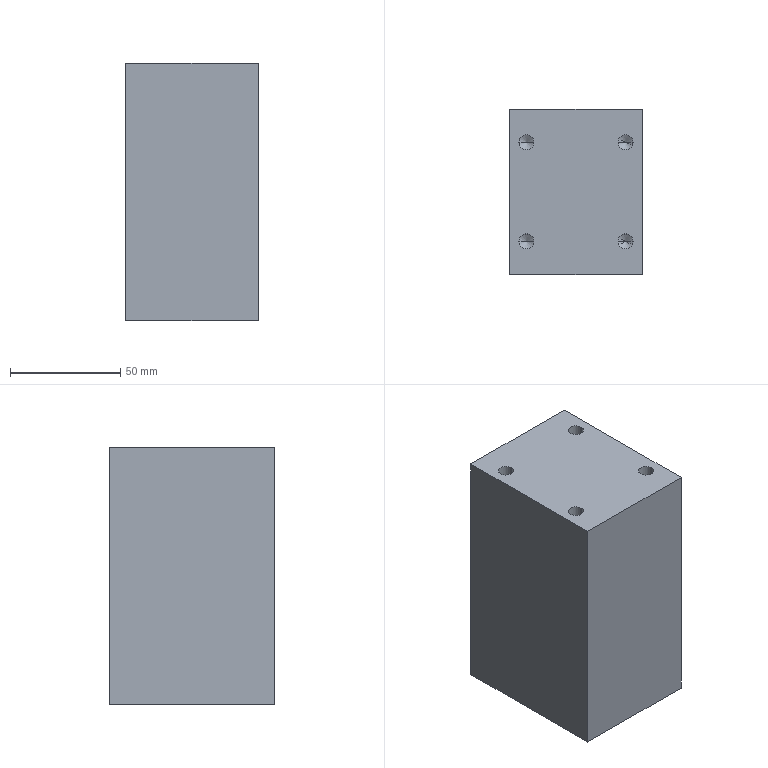Part | STEP file | Part 1^New head | 1 solid | 22 faces | box 60 x 75 x 117 mm | volume 523169 mm3 | cylinder 8 | cone 8 | plane 6 | commonest cylinder face diameters 6.8 x8
STEP:
#1=CARTESIAN_POINT('',(-75.9,-22.5,94.75));
#2=VERTEX_POINT('',#1);
#3=CARTESIAN_POINT('',(-69.1,-22.5,94.75));
#4=VERTEX_POINT('',#3);
#5=CARTESIAN_POINT('',(-72.5,-22.5,94.75));
#6=DIRECTION('',(0.,0.,1.));
#7=DIRECTION('',(1.,0.,0.));
#8=AXIS2_PLACEMENT_3D('',#5,#6,#7);
#9=CIRCLE('',#8,3.4);
#10=EDGE_CURVE('',#2,#4,#9,.T.);
#11=ORIENTED_EDGE('',*,*,#10,.F.);
#12=CARTESIAN_POINT('',(-75.9,-22.5,117.));
#13=VERTEX_POINT('',#12);
#14=CARTESIAN_POINT('',(-75.9,-22.5,117.));
#15=DIRECTION('',(0.,0.,1.));
#16=VECTOR('',#15,1000.);
#17=LINE('',#14,#16);
#18=EDGE_CURVE('',#2,#13,#17,.T.);
#19=ORIENTED_EDGE('',*,*,#18,.T.);
#20=CARTESIAN_POINT('',(-69.1,-22.5,117.));
#21=VERTEX_POINT('',#20);
#22=CARTESIAN_POINT('',(-72.5,-22.5,117.));
#23=DIRECTION('',(0.,0.,1.));
#24=DIRECTION('',(1.,0.,0.));
#25=AXIS2_PLACEMENT_3D('',#22,#23,#24);
#26=CIRCLE('',#25,3.4);
#27=EDGE_CURVE('',#13,#21,#26,.T.);
#28=ORIENTED_EDGE('',*,*,#27,.T.);
#29=CARTESIAN_POINT('',(-69.1,-22.5,117.));
#30=DIRECTION('',(0.,0.,1.));
#31=VECTOR('',#30,1000.);
#32=LINE('',#29,#31);
#33=EDGE_CURVE('',#4,#21,#32,.T.);
#34=ORIENTED_EDGE('',*,*,#33,.F.);
#35=EDGE_LOOP('',(#11,#19,#28,#34));
#36=FACE_OUTER_BOUND('',#35,.T.);
#37=CARTESIAN_POINT('',(-72.5,-22.5,117.));
#38=DIRECTION('',(0.,0.,1.));
#39=DIRECTION('',(1.,0.,0.));
#40=AXIS2_PLACEMENT_3D('',#37,#38,#39);
#41=CYLINDRICAL_SURFACE('',#40,3.4);
#42=ADVANCED_FACE('',(#36),#41,.F.);
#43=CARTESIAN_POINT('',(-72.5,-22.5,92.707));
#44=VERTEX_POINT('',#43);
#45=CARTESIAN_POINT('',(-69.1,-22.5,94.75));
#46=DIRECTION('',(0.8572,0.,0.515));
#47=VECTOR('',#46,1000.);
#48=LINE('',#45,#47);
#49=EDGE_CURVE('',#44,#4,#48,.T.);
#50=ORIENTED_EDGE('',*,*,#49,.F.);
#51=CARTESIAN_POINT('',(-75.9,-22.5,94.75));
#52=DIRECTION('',(-0.8572,0.,0.515));
#53=VECTOR('',#52,1000.);
#54=LINE('',#51,#53);
#55=EDGE_CURVE('',#44,#2,#54,.T.);
#56=ORIENTED_EDGE('',*,*,#55,.T.);
#57=ORIENTED_EDGE('',*,*,#10,.T.);
#58=EDGE_LOOP('',(#50,#56,#57));
#59=FACE_OUTER_BOUND('',#58,.T.);
#60=CARTESIAN_POINT('',(-72.5,-22.5,94.75));
#61=DIRECTION('',(0.,0.,1.));
#62=DIRECTION('',(1.,0.,0.));
#63=AXIS2_PLACEMENT_3D('',#60,#61,#62);
#64=CONICAL_SURFACE('',#63,3.4,1.03);
#65=ADVANCED_FACE('',(#59),#64,.F.);
#66=CARTESIAN_POINT('',(-75.9,22.5,94.75));
#67=VERTEX_POINT('',#66);
#68=CARTESIAN_POINT('',(-69.1,22.5,94.75));
#69=VERTEX_POINT('',#68);
#70=CARTESIAN_POINT('',(-72.5,22.5,94.75));
#71=DIRECTION('',(0.,0.,1.));
#72=DIRECTION('',(1.,0.,0.));
#73=AXIS2_PLACEMENT_3D('',#70,#71,#72);
#74=CIRCLE('',#73,3.4);
#75=EDGE_CURVE('',#67,#69,#74,.T.);
#76=ORIENTED_EDGE('',*,*,#75,.F.);
#77=CARTESIAN_POINT('',(-75.9,22.5,117.));
#78=VERTEX_POINT('',#77);
#79=CARTESIAN_POINT('',(-75.9,22.5,117.));
#80=DIRECTION('',(0.,0.,1.));
#81=VECTOR('',#80,1000.);
#82=LINE('',#79,#81);
#83=EDGE_CURVE('',#67,#78,#82,.T.);
#84=ORIENTED_EDGE('',*,*,#83,.T.);
#85=CARTESIAN_POINT('',(-69.1,22.5,117.));
#86=VERTEX_POINT('',#85);
#87=CARTESIAN_POINT('',(-72.5,22.5,117.));
#88=DIRECTION('',(0.,0.,1.));
#89=DIRECTION('',(1.,0.,0.));
#90=AXIS2_PLACEMENT_3D('',#87,#88,#89);
#91=CIRCLE('',#90,3.4);
#92=EDGE_CURVE('',#78,#86,#91,.T.);
#93=ORIENTED_EDGE('',*,*,#92,.T.);
#94=CARTESIAN_POINT('',(-69.1,22.5,117.));
#95=DIRECTION('',(0.,0.,1.));
#96=VECTOR('',#95,1000.);
#97=LINE('',#94,#96);
#98=EDGE_CURVE('',#69,#86,#97,.T.);
#99=ORIENTED_EDGE('',*,*,#98,.F.);
#100=EDGE_LOOP('',(#76,#84,#93,#99));
#101=FACE_OUTER_BOUND('',#100,.T.);
#102=CARTESIAN_POINT('',(-72.5,22.5,117.));
#103=DIRECTION('',(0.,0.,1.));
#104=DIRECTION('',(1.,0.,0.));
#105=AXIS2_PLACEMENT_3D('',#102,#103,#104);
#106=CYLINDRICAL_SURFACE('',#105,3.4);
#107=ADVANCED_FACE('',(#101),#106,.F.);
#108=CARTESIAN_POINT('',(-72.5,22.5,92.707));
#109=VERTEX_POINT('',#108);
#110=CARTESIAN_POINT('',(-69.1,22.5,94.75));
#111=DIRECTION('',(0.8572,0.,0.515));
#112=VECTOR('',#111,1000.);
#113=LINE('',#110,#112);
#114=EDGE_CURVE('',#109,#69,#113,.T.);
#115=ORIENTED_EDGE('',*,*,#114,.F.);
#116=CARTESIAN_POINT('',(-75.9,22.5,94.75));
#117=DIRECTION('',(-0.8572,0.,0.515));
#118=VECTOR('',#117,1000.);
#119=LINE('',#116,#118);
#120=EDGE_CURVE('',#109,#67,#119,.T.);
#121=ORIENTED_EDGE('',*,*,#120,.T.);
#122=ORIENTED_EDGE('',*,*,#75,.T.);
#123=EDGE_LOOP('',(#115,#121,#122));
#124=FACE_OUTER_BOUND('',#123,.T.);
#125=CARTESIAN_POINT('',(-72.5,22.5,94.75));
#126=DIRECTION('',(0.,0.,1.));
#127=DIRECTION('',(1.,0.,0.));
#128=AXIS2_PLACEMENT_3D('',#125,#126,#127);
#129=CONICAL_SURFACE('',#128,3.4,1.03);
#130=ADVANCED_FACE('',(#124),#129,.F.);
#131=CARTESIAN_POINT('',(-30.9,22.5,94.75));
#132=VERTEX_POINT('',#131);
#133=CARTESIAN_POINT('',(-24.1,22.5,94.75));
#134=VERTEX_POINT('',#133);
#135=CARTESIAN_POINT('',(-27.5,22.5,94.75));
#136=DIRECTION('',(0.,0.,1.));
#137=DIRECTION('',(1.,0.,0.));
#138=AXIS2_PLACEMENT_3D('',#135,#136,#137);
#139=CIRCLE('',#138,3.4);
#140=EDGE_CURVE('',#132,#134,#139,.T.);
#141=ORIENTED_EDGE('',*,*,#140,.F.);
#142=CARTESIAN_POINT('',(-30.9,22.5,117.));
#143=VERTEX_POINT('',#142);
#144=CARTESIAN_POINT('',(-30.9,22.5,117.));
#145=DIRECTION('',(0.,0.,1.));
#146=VECTOR('',#145,1000.);
#147=LINE('',#144,#146);
#148=EDGE_CURVE('',#132,#143,#147,.T.);
#149=ORIENTED_EDGE('',*,*,#148,.T.);
#150=CARTESIAN_POINT('',(-24.1,22.5,117.));
#151=VERTEX_POINT('',#150);
#152=CARTESIAN_POINT('',(-27.5,22.5,117.));
#153=DIRECTION('',(0.,0.,1.));
#154=DIRECTION('',(1.,0.,0.));
#155=AXIS2_PLACEMENT_3D('',#152,#153,#154);
#156=CIRCLE('',#155,3.4);
#157=EDGE_CURVE('',#143,#151,#156,.T.);
#158=ORIENTED_EDGE('',*,*,#157,.T.);
#159=CARTESIAN_POINT('',(-24.1,22.5,117.));
#160=DIRECTION('',(0.,0.,1.));
#161=VECTOR('',#160,1000.);
#162=LINE('',#159,#161);
#163=EDGE_CURVE('',#134,#151,#162,.T.);
#164=ORIENTED_EDGE('',*,*,#163,.F.);
#165=EDGE_LOOP('',(#141,#149,#158,#164));
#166=FACE_OUTER_BOUND('',#165,.T.);
#167=CARTESIAN_POINT('',(-27.5,22.5,117.));
#168=DIRECTION('',(0.,0.,1.));
#169=DIRECTION('',(1.,0.,0.));
#170=AXIS2_PLACEMENT_3D('',#167,#168,#169);
#171=CYLINDRICAL_SURFACE('',#170,3.4);
#172=ADVANCED_FACE('',(#166),#171,.F.);
#173=CARTESIAN_POINT('',(-27.5,22.5,92.707));
#174=VERTEX_POINT('',#173);
#175=CARTESIAN_POINT('',(-24.1,22.5,94.75));
#176=DIRECTION('',(0.8572,0.,0.515));
#177=VECTOR('',#176,1000.);
#178=LINE('',#175,#177);
#179=EDGE_CURVE('',#174,#134,#178,.T.);
#180=ORIENTED_EDGE('',*,*,#179,.F.);
#181=CARTESIAN_POINT('',(-30.9,22.5,94.75));
#182=DIRECTION('',(-0.8572,0.,0.515));
#183=VECTOR('',#182,1000.);
#184=LINE('',#181,#183);
#185=EDGE_CURVE('',#174,#132,#184,.T.);
#186=ORIENTED_EDGE('',*,*,#185,.T.);
#187=ORIENTED_EDGE('',*,*,#140,.T.);
#188=EDGE_LOOP('',(#180,#186,#187));
#189=FACE_OUTER_BOUND('',#188,.T.);
#190=CARTESIAN_POINT('',(-27.5,22.5,94.75));
#191=DIRECTION('',(0.,0.,1.));
#192=DIRECTION('',(1.,0.,0.));
#193=AXIS2_PLACEMENT_3D('',#190,#191,#192);
#194=CONICAL_SURFACE('',#193,3.4,1.03);
#195=ADVANCED_FACE('',(#189),#194,.F.);
#196=CARTESIAN_POINT('',(-30.9,-22.5,94.75));
#197=VERTEX_POINT('',#196);
#198=CARTESIAN_POINT('',(-24.1,-22.5,94.75));
#199=VERTEX_POINT('',#198);
#200=CARTESIAN_POINT('',(-27.5,-22.5,94.75));
#201=DIRECTION('',(0.,0.,1.));
#202=DIRECTION('',(1.,0.,0.));
#203=AXIS2_PLACEMENT_3D('',#200,#201,#202);
#204=CIRCLE('',#203,3.4);
#205=EDGE_CURVE('',#197,#199,#204,.T.);
#206=ORIENTED_EDGE('',*,*,#205,.F.);
#207=CARTESIAN_POINT('',(-30.9,-22.5,117.));
#208=VERTEX_POINT('',#207);
#209=CARTESIAN_POINT('',(-30.9,-22.5,117.));
#210=DIRECTION('',(0.,0.,1.));
#211=VECTOR('',#210,1000.);
#212=LINE('',#209,#211);
#213=EDGE_CURVE('',#197,#208,#212,.T.);
#214=ORIENTED_EDGE('',*,*,#213,.T.);
#215=CARTESIAN_POINT('',(-24.1,-22.5,117.));
#216=VERTEX_POINT('',#215);
#217=CARTESIAN_POINT('',(-27.5,-22.5,117.));
#218=DIRECTION('',(0.,0.,1.));
#219=DIRECTION('',(1.,0.,0.));
#220=AXIS2_PLACEMENT_3D('',#217,#218,#219);
#221=CIRCLE('',#220,3.4);
#222=EDGE_CURVE('',#208,#216,#221,.T.);
#223=ORIENTED_EDGE('',*,*,#222,.T.);
#224=CARTESIAN_POINT('',(-24.1,-22.5,117.));
#225=DIRECTION('',(0.,0.,1.));
#226=VECTOR('',#225,1000.);
#227=LINE('',#224,#226);
#228=EDGE_CURVE('',#199,#216,#227,.T.);
#229=ORIENTED_EDGE('',*,*,#228,.F.);
#230=EDGE_LOOP('',(#206,#214,#223,#229));
#231=FACE_OUTER_BOUND('',#230,.T.);
#232=CARTESIAN_POINT('',(-27.5,-22.5,117.));
#233=DIRECTION('',(0.,0.,1.));
#234=DIRECTION('',(1.,0.,0.));
#235=AXIS2_PLACEMENT_3D('',#232,#233,#234);
#236=CYLINDRICAL_SURFACE('',#235,3.4);
#237=ADVANCED_FACE('',(#231),#236,.F.);
#238=CARTESIAN_POINT('',(-27.5,-22.5,92.707));
#239=VERTEX_POINT('',#238);
#240=CARTESIAN_POINT('',(-24.1,-22.5,94.75));
#241=DIRECTION('',(0.8572,0.,0.515));
#242=VECTOR('',#241,1000.);
#243=LINE('',#240,#242);
#244=EDGE_CURVE('',#239,#199,#243,.T.);
#245=ORIENTED_EDGE('',*,*,#244,.F.);
#246=CARTESIAN_POINT('',(-30.9,-22.5,94.75));
#247=DIRECTION('',(-0.8572,0.,0.515));
#248=VECTOR('',#247,1000.);
#249=LINE('',#246,#248);
#250=EDGE_CURVE('',#239,#197,#249,.T.);
#251=ORIENTED_EDGE('',*,*,#250,.T.);
#252=ORIENTED_EDGE('',*,*,#205,.T.);
#253=EDGE_LOOP('',(#245,#251,#252));
#254=FACE_OUTER_BOUND('',#253,.T.);
#255=CARTESIAN_POINT('',(-27.5,-22.5,94.75));
#256=DIRECTION('',(0.,0.,1.));
#257=DIRECTION('',(1.,0.,0.));
#258=AXIS2_PLACEMENT_3D('',#255,#256,#257);
#259=CONICAL_SURFACE('',#258,3.4,1.03);
#260=ADVANCED_FACE('',(#254),#259,.F.);
#261=CARTESIAN_POINT('',(-80.,37.5,0.));
#262=VERTEX_POINT('',#261);
#263=CARTESIAN_POINT('',(-80.,-37.5,0.));
#264=VERTEX_POINT('',#263);
#265=CARTESIAN_POINT('',(-80.,37.5,0.));
#266=DIRECTION('',(0.,-1.,0.));
#267=VECTOR('',#266,1000.);
#268=LINE('',#265,#267);
#269=EDGE_CURVE('',#262,#264,#268,.T.);
#270=ORIENTED_EDGE('',*,*,#269,.T.);
#271=CARTESIAN_POINT('',(-80.,-37.5,117.));
#272=VERTEX_POINT('',#271);
#273=CARTESIAN_POINT('',(-80.,-37.5,117.));
#274=DIRECTION('',(0.,0.,-1.));
#275=VECTOR('',#274,1000.);
#276=LINE('',#273,#275);
#277=EDGE_CURVE('',#272,#264,#276,.T.);
#278=ORIENTED_EDGE('',*,*,#277,.F.);
#279=CARTESIAN_POINT('',(-80.,37.5,117.));
#280=VERTEX_POINT('',#279);
#281=CARTESIAN_POINT('',(-80.,37.5,117.));
#282=DIRECTION('',(0.,-1.,0.));
#283=VECTOR('',#282,1000.);
#284=LINE('',#281,#283);
#285=EDGE_CURVE('',#280,#272,#284,.T.);
#286=ORIENTED_EDGE('',*,*,#285,.F.);
#287=CARTESIAN_POINT('',(-80.,37.5,117.));
#288=DIRECTION('',(0.,0.,-1.));
#289=VECTOR('',#288,1000.);
#290=LINE('',#287,#289);
#291=EDGE_CURVE('',#280,#262,#290,.T.);
#292=ORIENTED_EDGE('',*,*,#291,.T.);
#293=EDGE_LOOP('',(#270,#278,#286,#292));
#294=FACE_OUTER_BOUND('',#293,.T.);
#295=CARTESIAN_POINT('',(-80.,37.5,117.));
#296=DIRECTION('',(1.,0.,0.));
#297=DIRECTION('',(0.,1.,0.));
#298=AXIS2_PLACEMENT_3D('',#295,#296,#297);
#299=PLANE('',#298);
#300=ADVANCED_FACE('',(#294),#299,.F.);
#301=CARTESIAN_POINT('',(-20.,-37.5,0.));
#302=VERTEX_POINT('',#301);
#303=CARTESIAN_POINT('',(-80.,-37.5,0.));
#304=DIRECTION('',(1.,0.,0.));
#305=VECTOR('',#304,1000.);
#306=LINE('',#303,#305);
#307=EDGE_CURVE('',#264,#302,#306,.T.);
#308=ORIENTED_EDGE('',*,*,#307,.T.);
#309=CARTESIAN_POINT('',(-20.,-37.5,117.));
#310=VERTEX_POINT('',#309);
#311=CARTESIAN_POINT('',(-20.,-37.5,117.));
#312=DIRECTION('',(0.,0.,-1.));
#313=VECTOR('',#312,1000.);
#314=LINE('',#311,#313);
#315=EDGE_CURVE('',#310,#302,#314,.T.);
#316=ORIENTED_EDGE('',*,*,#315,.F.);
#317=CARTESIAN_POINT('',(-80.,-37.5,117.));
#318=DIRECTION('',(1.,0.,0.));
#319=VECTOR('',#318,1000.);
#320=LINE('',#317,#319);
#321=EDGE_CURVE('',#272,#310,#320,.T.);
#322=ORIENTED_EDGE('',*,*,#321,.F.);
#323=ORIENTED_EDGE('',*,*,#277,.T.);
#324=EDGE_LOOP('',(#308,#316,#322,#323));
#325=FACE_OUTER_BOUND('',#324,.T.);
#326=CARTESIAN_POINT('',(-80.,-37.5,117.));
#327=DIRECTION('',(0.,1.,0.));
#328=DIRECTION('',(-1.,0.,0.));
#329=AXIS2_PLACEMENT_3D('',#326,#327,#328);
#330=PLANE('',#329);
#331=ADVANCED_FACE('',(#325),#330,.F.);
#332=CARTESIAN_POINT('',(-20.,37.5,0.));
#333=VERTEX_POINT('',#332);
#334=CARTESIAN_POINT('',(-20.,37.5,0.));
#335=DIRECTION('',(0.,1.,0.));
#336=VECTOR('',#335,1000.);
#337=LINE('',#334,#336);
#338=EDGE_CURVE('',#302,#333,#337,.T.);
#339=ORIENTED_EDGE('',*,*,#338,.T.);
#340=CARTESIAN_POINT('',(-20.,37.5,117.));
#341=VERTEX_POINT('',#340);
#342=CARTESIAN_POINT('',(-20.,37.5,117.));
#343=DIRECTION('',(0.,0.,-1.));
#344=VECTOR('',#343,1000.);
#345=LINE('',#342,#344);
#346=EDGE_CURVE('',#341,#333,#345,.T.);
#347=ORIENTED_EDGE('',*,*,#346,.F.);
#348=CARTESIAN_POINT('',(-20.,37.5,117.));
#349=DIRECTION('',(0.,1.,0.));
#350=VECTOR('',#349,1000.);
#351=LINE('',#348,#350);
#352=EDGE_CURVE('',#310,#341,#351,.T.);
#353=ORIENTED_EDGE('',*,*,#352,.F.);
#354=ORIENTED_EDGE('',*,*,#315,.T.);
#355=EDGE_LOOP('',(#339,#347,#353,#354));
#356=FACE_OUTER_BOUND('',#355,.T.);
#357=CARTESIAN_POINT('',(-20.,37.5,117.));
#358=DIRECTION('',(-1.,0.,0.));
#359=DIRECTION('',(0.,-1.,0.));
#360=AXIS2_PLACEMENT_3D('',#357,#358,#359);
#361=PLANE('',#360);
#362=ADVANCED_FACE('',(#356),#361,.F.);
#363=CARTESIAN_POINT('',(-80.,37.5,0.));
#364=DIRECTION('',(-1.,0.,0.));
#365=VECTOR('',#364,1000.);
#366=LINE('',#363,#365);
#367=EDGE_CURVE('',#333,#262,#366,.T.);
#368=ORIENTED_EDGE('',*,*,#367,.T.);
#369=ORIENTED_EDGE('',*,*,#291,.F.);
#370=CARTESIAN_POINT('',(-80.,37.5,117.));
#371=DIRECTION('',(-1.,0.,0.));
#372=VECTOR('',#371,1000.);
#373=LINE('',#370,#372);
#374=EDGE_CURVE('',#341,#280,#373,.T.);
#375=ORIENTED_EDGE('',*,*,#374,.F.);
#376=ORIENTED_EDGE('',*,*,#346,.T.);
#377=EDGE_LOOP('',(#368,#369,#375,#376));
#378=FACE_OUTER_BOUND('',#377,.T.);
#379=CARTESIAN_POINT('',(-80.,37.5,117.));
#380=DIRECTION('',(0.,-1.,0.));
#381=DIRECTION('',(0.,0.,-1.));
#382=AXIS2_PLACEMENT_3D('',#379,#380,#381);
#383=PLANE('',#382);
#384=ADVANCED_FACE('',(#378),#383,.F.);
#385=CARTESIAN_POINT('',(-72.5,-22.5,117.));
#386=DIRECTION('',(0.,0.,1.));
#387=DIRECTION('',(1.,0.,0.));
#388=AXIS2_PLACEMENT_3D('',#385,#386,#387);
#389=CIRCLE('',#388,3.4);
#390=EDGE_CURVE('',#21,#13,#389,.T.);
#391=ORIENTED_EDGE('',*,*,#390,.F.);
#392=ORIENTED_EDGE('',*,*,#27,.F.);
#393=EDGE_LOOP('',(#391,#392));
#394=FACE_BOUND('',#393,.T.);
#395=CARTESIAN_POINT('',(-72.5,22.5,117.));
#396=DIRECTION('',(0.,0.,1.));
#397=DIRECTION('',(1.,0.,0.));
#398=AXIS2_PLACEMENT_3D('',#395,#396,#397);
#399=CIRCLE('',#398,3.4);
#400=EDGE_CURVE('',#86,#78,#399,.T.);
#401=ORIENTED_EDGE('',*,*,#400,.F.);
#402=ORIENTED_EDGE('',*,*,#92,.F.);
#403=EDGE_LOOP('',(#401,#402));
#404=FACE_BOUND('',#403,.T.);
#405=CARTESIAN_POINT('',(-27.5,22.5,117.));
#406=DIRECTION('',(0.,0.,1.));
#407=DIRECTION('',(1.,0.,0.));
#408=AXIS2_PLACEMENT_3D('',#405,#406,#407);
#409=CIRCLE('',#408,3.4);
#410=EDGE_CURVE('',#151,#143,#409,.T.);
#411=ORIENTED_EDGE('',*,*,#410,.F.);
#412=ORIENTED_EDGE('',*,*,#157,.F.);
#413=EDGE_LOOP('',(#411,#412));
#414=FACE_BOUND('',#413,.T.);
#415=CARTESIAN_POINT('',(-27.5,-22.5,117.));
#416=DIRECTION('',(0.,0.,1.));
#417=DIRECTION('',(1.,0.,0.));
#418=AXIS2_PLACEMENT_3D('',#415,#416,#417);
#419=CIRCLE('',#418,3.4);
#420=EDGE_CURVE('',#216,#208,#419,.T.);
#421=ORIENTED_EDGE('',*,*,#420,.F.);
#422=ORIENTED_EDGE('',*,*,#222,.F.);
#423=EDGE_LOOP('',(#421,#422));
#424=FACE_BOUND('',#423,.T.);
#425=ORIENTED_EDGE('',*,*,#285,.T.);
#426=ORIENTED_EDGE('',*,*,#321,.T.);
#427=ORIENTED_EDGE('',*,*,#352,.T.);
#428=ORIENTED_EDGE('',*,*,#374,.T.);
#429=EDGE_LOOP('',(#425,#426,#427,#428));
#430=FACE_OUTER_BOUND('',#429,.T.);
#431=CARTESIAN_POINT('',(0.,0.,117.));
#432=DIRECTION('',(0.,0.,1.));
#433=DIRECTION('',(1.,0.,0.));
#434=AXIS2_PLACEMENT_3D('',#431,#432,#433);
#435=PLANE('',#434);
#436=ADVANCED_FACE('',(#394,#404,#414,#424,#430),#435,.T.);
#437=ORIENTED_EDGE('',*,*,#269,.F.);
#438=ORIENTED_EDGE('',*,*,#367,.F.);
#439=ORIENTED_EDGE('',*,*,#338,.F.);
#440=ORIENTED_EDGE('',*,*,#307,.F.);
#441=EDGE_LOOP('',(#437,#438,#439,#440));
#442=FACE_OUTER_BOUND('',#441,.T.);
#443=CARTESIAN_POINT('',(0.,0.,0.));
#444=DIRECTION('',(0.,0.,1.));
#445=DIRECTION('',(1.,0.,0.));
#446=AXIS2_PLACEMENT_3D('',#443,#444,#445);
#447=PLANE('',#446);
#448=ADVANCED_FACE('',(#442),#447,.F.);
#449=ORIENTED_EDGE('',*,*,#250,.F.);
#450=ORIENTED_EDGE('',*,*,#244,.T.);
#451=CARTESIAN_POINT('',(-27.5,-22.5,94.75));
#452=DIRECTION('',(0.,0.,1.));
#453=DIRECTION('',(1.,0.,0.));
#454=AXIS2_PLACEMENT_3D('',#451,#452,#453);
#455=CIRCLE('',#454,3.4);
#456=EDGE_CURVE('',#199,#197,#455,.T.);
#457=ORIENTED_EDGE('',*,*,#456,.T.);
#458=EDGE_LOOP('',(#449,#450,#457));
#459=FACE_OUTER_BOUND('',#458,.T.);
#460=CARTESIAN_POINT('',(-27.5,-22.5,94.75));
#461=DIRECTION('',(0.,0.,1.));
#462=DIRECTION('',(1.,0.,0.));
#463=AXIS2_PLACEMENT_3D('',#460,#461,#462);
#464=CONICAL_SURFACE('',#463,3.4,1.03);
#465=ADVANCED_FACE('',(#459),#464,.F.);
#466=ORIENTED_EDGE('',*,*,#213,.F.);
#467=ORIENTED_EDGE('',*,*,#456,.F.);
#468=ORIENTED_EDGE('',*,*,#228,.T.);
#469=ORIENTED_EDGE('',*,*,#420,.T.);
#470=EDGE_LOOP('',(#466,#467,#468,#469));
#471=FACE_OUTER_BOUND('',#470,.T.);
#472=CARTESIAN_POINT('',(-27.5,-22.5,117.));
#473=DIRECTION('',(0.,0.,1.));
#474=DIRECTION('',(1.,0.,0.));
#475=AXIS2_PLACEMENT_3D('',#472,#473,#474);
#476=CYLINDRICAL_SURFACE('',#475,3.4);
#477=ADVANCED_FACE('',(#471),#476,.F.);
#478=ORIENTED_EDGE('',*,*,#185,.F.);
#479=ORIENTED_EDGE('',*,*,#179,.T.);
#480=CARTESIAN_POINT('',(-27.5,22.5,94.75));
#481=DIRECTION('',(0.,0.,1.));
#482=DIRECTION('',(1.,0.,0.));
#483=AXIS2_PLACEMENT_3D('',#480,#481,#482);
#484=CIRCLE('',#483,3.4);
#485=EDGE_CURVE('',#134,#132,#484,.T.);
#486=ORIENTED_EDGE('',*,*,#485,.T.);
#487=EDGE_LOOP('',(#478,#479,#486));
#488=FACE_OUTER_BOUND('',#487,.T.);
#489=CARTESIAN_POINT('',(-27.5,22.5,94.75));
#490=DIRECTION('',(0.,0.,1.));
#491=DIRECTION('',(1.,0.,0.));
#492=AXIS2_PLACEMENT_3D('',#489,#490,#491);
#493=CONICAL_SURFACE('',#492,3.4,1.03);
#494=ADVANCED_FACE('',(#488),#493,.F.);
#495=ORIENTED_EDGE('',*,*,#148,.F.);
#496=ORIENTED_EDGE('',*,*,#485,.F.);
#497=ORIENTED_EDGE('',*,*,#163,.T.);
#498=ORIENTED_EDGE('',*,*,#410,.T.);
#499=EDGE_LOOP('',(#495,#496,#497,#498));
#500=FACE_OUTER_BOUND('',#499,.T.);
#501=CARTESIAN_POINT('',(-27.5,22.5,117.));
#502=DIRECTION('',(0.,0.,1.));
#503=DIRECTION('',(1.,0.,0.));
#504=AXIS2_PLACEMENT_3D('',#501,#502,#503);
#505=CYLINDRICAL_SURFACE('',#504,3.4);
#506=ADVANCED_FACE('',(#500),#505,.F.);
#507=ORIENTED_EDGE('',*,*,#120,.F.);
#508=ORIENTED_EDGE('',*,*,#114,.T.);
#509=CARTESIAN_POINT('',(-72.5,22.5,94.75));
#510=DIRECTION('',(0.,0.,1.));
#511=DIRECTION('',(1.,0.,0.));
#512=AXIS2_PLACEMENT_3D('',#509,#510,#511);
#513=CIRCLE('',#512,3.4);
#514=EDGE_CURVE('',#69,#67,#513,.T.);
#515=ORIENTED_EDGE('',*,*,#514,.T.);
#516=EDGE_LOOP('',(#507,#508,#515));
#517=FACE_OUTER_BOUND('',#516,.T.);
#518=CARTESIAN_POINT('',(-72.5,22.5,94.75));
#519=DIRECTION('',(0.,0.,1.));
#520=DIRECTION('',(1.,0.,0.));
#521=AXIS2_PLACEMENT_3D('',#518,#519,#520);
#522=CONICAL_SURFACE('',#521,3.4,1.03);
#523=ADVANCED_FACE('',(#517),#522,.F.);
#524=ORIENTED_EDGE('',*,*,#83,.F.);
#525=ORIENTED_EDGE('',*,*,#514,.F.);
#526=ORIENTED_EDGE('',*,*,#98,.T.);
#527=ORIENTED_EDGE('',*,*,#400,.T.);
#528=EDGE_LOOP('',(#524,#525,#526,#527));
#529=FACE_OUTER_BOUND('',#528,.T.);
#530=CARTESIAN_POINT('',(-72.5,22.5,117.));
#531=DIRECTION('',(0.,0.,1.));
#532=DIRECTION('',(1.,0.,0.));
#533=AXIS2_PLACEMENT_3D('',#530,#531,#532);
#534=CYLINDRICAL_SURFACE('',#533,3.4);
#535=ADVANCED_FACE('',(#529),#534,.F.);
#536=ORIENTED_EDGE('',*,*,#55,.F.);
#537=ORIENTED_EDGE('',*,*,#49,.T.);
#538=CARTESIAN_POINT('',(-72.5,-22.5,94.75));
#539=DIRECTION('',(0.,0.,1.));
#540=DIRECTION('',(1.,0.,0.));
#541=AXIS2_PLACEMENT_3D('',#538,#539,#540);
#542=CIRCLE('',#541,3.4);
#543=EDGE_CURVE('',#4,#2,#542,.T.);
#544=ORIENTED_EDGE('',*,*,#543,.T.);
#545=EDGE_LOOP('',(#536,#537,#544));
#546=FACE_OUTER_BOUND('',#545,.T.);
#547=CARTESIAN_POINT('',(-72.5,-22.5,94.75));
#548=DIRECTION('',(0.,0.,1.));
#549=DIRECTION('',(1.,0.,0.));
#550=AXIS2_PLACEMENT_3D('',#547,#548,#549);
#551=CONICAL_SURFACE('',#550,3.4,1.03);
#552=ADVANCED_FACE('',(#546),#551,.F.);
#553=ORIENTED_EDGE('',*,*,#18,.F.);
#554=ORIENTED_EDGE('',*,*,#543,.F.);
#555=ORIENTED_EDGE('',*,*,#33,.T.);
#556=ORIENTED_EDGE('',*,*,#390,.T.);
#557=EDGE_LOOP('',(#553,#554,#555,#556));
#558=FACE_OUTER_BOUND('',#557,.T.);
#559=CARTESIAN_POINT('',(-72.5,-22.5,117.));
#560=DIRECTION('',(0.,0.,1.));
#561=DIRECTION('',(1.,0.,0.));
#562=AXIS2_PLACEMENT_3D('',#559,#560,#561);
#563=CYLINDRICAL_SURFACE('',#562,3.4);
#564=ADVANCED_FACE('',(#558),#563,.F.);
#565=CLOSED_SHELL('',(#42,#65,#107,#130,#172,#195,#237,#260,#300,#331,#362,#384,#436,#448,#465,#477,#494,#506,#523,#535,#552,#564));
#566=MANIFOLD_SOLID_BREP('',#565);
#567=CARTESIAN_POINT('',(0.,0.,0.));
#568=DIRECTION('',(0.,0.,1.));
#569=DIRECTION('',(1.,0.,0.));
#570=AXIS2_PLACEMENT_3D('',#567,#568,#569);
#571=(LENGTH_UNIT()NAMED_UNIT(*)SI_UNIT(.MILLI.,.METRE.));
#572=UNCERTAINTY_MEASURE_WITH_UNIT(LENGTH_MEASURE(0.00001),#571,'','');
#573=(NAMED_UNIT(*)PLANE_ANGLE_UNIT()SI_UNIT($,.RADIAN.));
#574=(NAMED_UNIT(*)SI_UNIT($,.STERADIAN.)SOLID_ANGLE_UNIT());
#575=(GEOMETRIC_REPRESENTATION_CONTEXT(3)GLOBAL_UNCERTAINTY_ASSIGNED_CONTEXT((#572))GLOBAL_UNIT_ASSIGNED_CONTEXT((#571,#573,#574))REPRESENTATION_CONTEXT('',''));
#576=ADVANCED_BREP_SHAPE_REPRESENTATION('',(#566,#570),#575);